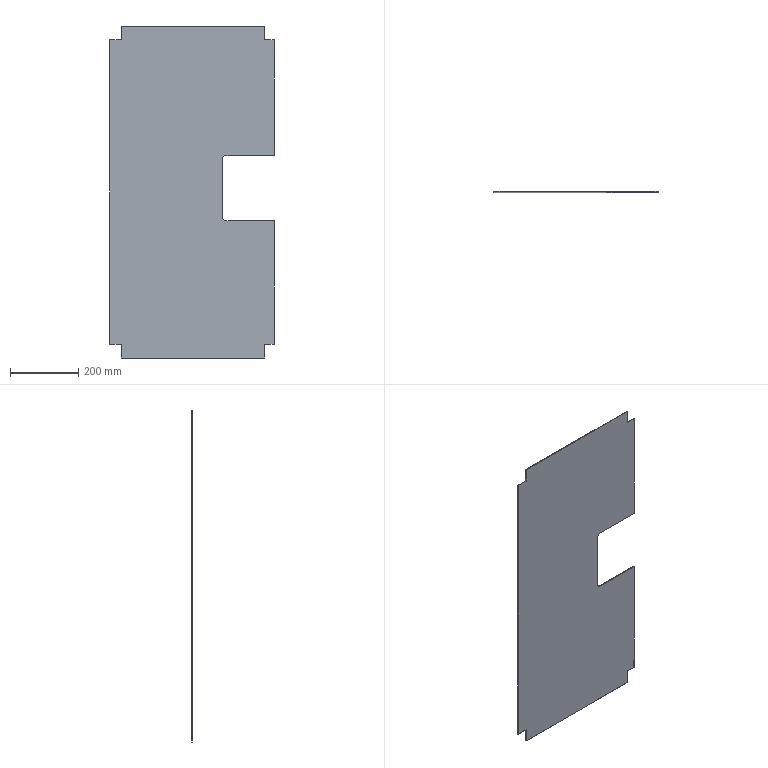Part | SolidWorks | features BaseBody 1 | 1 solid | 20 faces | box 480 x 1.5 x 970 mm | volume 648201 mm3 | plane 18 | cylinder 2 | commonest cylinder face diameters 20 x2
STEP:
#1=CARTESIAN_POINT('',(82.823,-1.5,-83.686));
#2=VERTEX_POINT('',#1);
#3=CARTESIAN_POINT('',(223.5,-1.5,-83.686));
#4=VERTEX_POINT('',#3);
#5=CARTESIAN_POINT('',(0.,-1.5,-83.686));
#6=DIRECTION('',(1.,0.,0.));
#7=VECTOR('',#6,1000.);
#8=LINE('',#5,#7);
#9=EDGE_CURVE('',#2,#4,#8,.T.);
#10=ORIENTED_EDGE('',*,*,#9,.F.);
#11=CARTESIAN_POINT('',(72.823,-1.5,-73.686));
#12=VERTEX_POINT('',#11);
#13=CARTESIAN_POINT('',(82.823,-1.5,-73.686));
#14=DIRECTION('',(0.,-1.,0.));
#15=DIRECTION('',(0.,0.,1.));
#16=AXIS2_PLACEMENT_3D('',#13,#14,#15);
#17=CIRCLE('',#16,10.);
#18=EDGE_CURVE('',#12,#2,#17,.T.);
#19=ORIENTED_EDGE('',*,*,#18,.F.);
#20=CARTESIAN_POINT('',(72.823,-1.5,96.314));
#21=VERTEX_POINT('',#20);
#22=CARTESIAN_POINT('',(72.823,-1.5,0.));
#23=DIRECTION('',(0.,0.,-1.));
#24=VECTOR('',#23,1000.);
#25=LINE('',#22,#24);
#26=EDGE_CURVE('',#21,#12,#25,.T.);
#27=ORIENTED_EDGE('',*,*,#26,.F.);
#28=CARTESIAN_POINT('',(82.823,-1.5,106.314));
#29=VERTEX_POINT('',#28);
#30=CARTESIAN_POINT('',(82.823,-1.5,96.314));
#31=DIRECTION('',(0.,-1.,0.));
#32=DIRECTION('',(0.,0.,1.));
#33=AXIS2_PLACEMENT_3D('',#30,#31,#32);
#34=CIRCLE('',#33,10.);
#35=EDGE_CURVE('',#29,#21,#34,.T.);
#36=ORIENTED_EDGE('',*,*,#35,.F.);
#37=CARTESIAN_POINT('',(223.5,-1.5,106.314));
#38=VERTEX_POINT('',#37);
#39=CARTESIAN_POINT('',(0.,-1.5,106.314));
#40=DIRECTION('',(-1.,0.,0.));
#41=VECTOR('',#40,1000.);
#42=LINE('',#39,#41);
#43=EDGE_CURVE('',#38,#29,#42,.T.);
#44=ORIENTED_EDGE('',*,*,#43,.F.);
#45=CARTESIAN_POINT('',(223.5,-1.5,445.));
#46=VERTEX_POINT('',#45);
#47=CARTESIAN_POINT('',(223.5,-1.5,0.));
#48=DIRECTION('',(0.,0.,-1.));
#49=VECTOR('',#48,1000.);
#50=LINE('',#47,#49);
#51=EDGE_CURVE('',#46,#38,#50,.T.);
#52=ORIENTED_EDGE('',*,*,#51,.F.);
#53=CARTESIAN_POINT('',(195.5,-1.5,445.));
#54=VERTEX_POINT('',#53);
#55=CARTESIAN_POINT('',(0.,-1.5,445.));
#56=DIRECTION('',(1.,0.,0.));
#57=VECTOR('',#56,1000.);
#58=LINE('',#55,#57);
#59=EDGE_CURVE('',#54,#46,#58,.T.);
#60=ORIENTED_EDGE('',*,*,#59,.F.);
#61=CARTESIAN_POINT('',(195.5,-1.5,485.));
#62=VERTEX_POINT('',#61);
#63=CARTESIAN_POINT('',(195.5,-1.5,0.));
#64=DIRECTION('',(0.,0.,-1.));
#65=VECTOR('',#64,1000.);
#66=LINE('',#63,#65);
#67=EDGE_CURVE('',#62,#54,#66,.T.);
#68=ORIENTED_EDGE('',*,*,#67,.F.);
#69=CARTESIAN_POINT('',(-223.5,-1.5,485.));
#70=VERTEX_POINT('',#69);
#71=CARTESIAN_POINT('',(0.,-1.5,485.));
#72=DIRECTION('',(1.,0.,0.));
#73=VECTOR('',#72,1000.);
#74=LINE('',#71,#73);
#75=EDGE_CURVE('',#70,#62,#74,.T.);
#76=ORIENTED_EDGE('',*,*,#75,.F.);
#77=CARTESIAN_POINT('',(-223.5,-1.5,445.));
#78=VERTEX_POINT('',#77);
#79=CARTESIAN_POINT('',(-223.5,-1.5,0.));
#80=DIRECTION('',(0.,0.,1.));
#81=VECTOR('',#80,1000.);
#82=LINE('',#79,#81);
#83=EDGE_CURVE('',#78,#70,#82,.T.);
#84=ORIENTED_EDGE('',*,*,#83,.F.);
#85=CARTESIAN_POINT('',(-256.5,-1.5,445.));
#86=VERTEX_POINT('',#85);
#87=CARTESIAN_POINT('',(0.,-1.5,445.));
#88=DIRECTION('',(1.,0.,0.));
#89=VECTOR('',#88,1000.);
#90=LINE('',#87,#89);
#91=EDGE_CURVE('',#86,#78,#90,.T.);
#92=ORIENTED_EDGE('',*,*,#91,.F.);
#93=CARTESIAN_POINT('',(-256.5,-1.5,-445.));
#94=VERTEX_POINT('',#93);
#95=CARTESIAN_POINT('',(-256.5,-1.5,0.));
#96=DIRECTION('',(0.,0.,1.));
#97=VECTOR('',#96,1000.);
#98=LINE('',#95,#97);
#99=EDGE_CURVE('',#94,#86,#98,.T.);
#100=ORIENTED_EDGE('',*,*,#99,.F.);
#101=CARTESIAN_POINT('',(-223.5,-1.5,-445.));
#102=VERTEX_POINT('',#101);
#103=CARTESIAN_POINT('',(0.,-1.5,-445.));
#104=DIRECTION('',(-1.,0.,0.));
#105=VECTOR('',#104,1000.);
#106=LINE('',#103,#105);
#107=EDGE_CURVE('',#102,#94,#106,.T.);
#108=ORIENTED_EDGE('',*,*,#107,.F.);
#109=CARTESIAN_POINT('',(-223.5,-1.5,-485.));
#110=VERTEX_POINT('',#109);
#111=CARTESIAN_POINT('',(-223.5,-1.5,0.));
#112=DIRECTION('',(0.,0.,1.));
#113=VECTOR('',#112,1000.);
#114=LINE('',#111,#113);
#115=EDGE_CURVE('',#110,#102,#114,.T.);
#116=ORIENTED_EDGE('',*,*,#115,.F.);
#117=CARTESIAN_POINT('',(195.5,-1.5,-485.));
#118=VERTEX_POINT('',#117);
#119=CARTESIAN_POINT('',(0.,-1.5,-485.));
#120=DIRECTION('',(-1.,0.,0.));
#121=VECTOR('',#120,1000.);
#122=LINE('',#119,#121);
#123=EDGE_CURVE('',#118,#110,#122,.T.);
#124=ORIENTED_EDGE('',*,*,#123,.F.);
#125=CARTESIAN_POINT('',(195.5,-1.5,-445.));
#126=VERTEX_POINT('',#125);
#127=CARTESIAN_POINT('',(195.5,-1.5,0.));
#128=DIRECTION('',(0.,0.,-1.));
#129=VECTOR('',#128,1000.);
#130=LINE('',#127,#129);
#131=EDGE_CURVE('',#126,#118,#130,.T.);
#132=ORIENTED_EDGE('',*,*,#131,.F.);
#133=CARTESIAN_POINT('',(223.5,-1.5,-445.));
#134=VERTEX_POINT('',#133);
#135=CARTESIAN_POINT('',(0.,-1.5,-445.));
#136=DIRECTION('',(-1.,0.,0.));
#137=VECTOR('',#136,1000.);
#138=LINE('',#135,#137);
#139=EDGE_CURVE('',#134,#126,#138,.T.);
#140=ORIENTED_EDGE('',*,*,#139,.F.);
#141=CARTESIAN_POINT('',(223.5,-1.5,0.));
#142=DIRECTION('',(0.,0.,-1.));
#143=VECTOR('',#142,1000.);
#144=LINE('',#141,#143);
#145=EDGE_CURVE('',#4,#134,#144,.T.);
#146=ORIENTED_EDGE('',*,*,#145,.F.);
#147=EDGE_LOOP('',(#10,#19,#27,#36,#44,#52,#60,#68,#76,#84,#92,#100,#108,#116,#124,#132,#140,#146));
#148=FACE_OUTER_BOUND('',#147,.T.);
#149=CARTESIAN_POINT('',(0.,-1.5,0.));
#150=DIRECTION('',(0.,1.,0.));
#151=DIRECTION('',(0.,0.,1.));
#152=AXIS2_PLACEMENT_3D('',#149,#150,#151);
#153=PLANE('',#152);
#154=ADVANCED_FACE('',(#148),#153,.F.);
#155=CARTESIAN_POINT('',(223.5,0.,-445.));
#156=VERTEX_POINT('',#155);
#157=CARTESIAN_POINT('',(223.5,-1.5,-445.));
#158=DIRECTION('',(0.,1.,0.));
#159=VECTOR('',#158,1000.);
#160=LINE('',#157,#159);
#161=EDGE_CURVE('',#134,#156,#160,.T.);
#162=ORIENTED_EDGE('',*,*,#161,.T.);
#163=CARTESIAN_POINT('',(223.5,0.,-83.686));
#164=VERTEX_POINT('',#163);
#165=CARTESIAN_POINT('',(223.5,0.,445.));
#166=DIRECTION('',(0.,0.,1.));
#167=VECTOR('',#166,1000.);
#168=LINE('',#165,#167);
#169=EDGE_CURVE('',#156,#164,#168,.T.);
#170=ORIENTED_EDGE('',*,*,#169,.T.);
#171=CARTESIAN_POINT('',(223.5,-1.5,-83.686));
#172=DIRECTION('',(0.,-1.,0.));
#173=VECTOR('',#172,1000.);
#174=LINE('',#171,#173);
#175=EDGE_CURVE('',#164,#4,#174,.T.);
#176=ORIENTED_EDGE('',*,*,#175,.T.);
#177=ORIENTED_EDGE('',*,*,#145,.T.);
#178=EDGE_LOOP('',(#162,#170,#176,#177));
#179=FACE_OUTER_BOUND('',#178,.T.);
#180=CARTESIAN_POINT('',(223.5,-1.5,445.));
#181=DIRECTION('',(1.,0.,0.));
#182=DIRECTION('',(0.,0.,-1.));
#183=AXIS2_PLACEMENT_3D('',#180,#181,#182);
#184=PLANE('',#183);
#185=ADVANCED_FACE('',(#179),#184,.T.);
#186=CARTESIAN_POINT('',(82.823,0.,-83.686));
#187=VERTEX_POINT('',#186);
#188=CARTESIAN_POINT('',(372.823,0.,-83.686));
#189=DIRECTION('',(1.,0.,0.));
#190=VECTOR('',#189,1000.);
#191=LINE('',#188,#190);
#192=EDGE_CURVE('',#187,#164,#191,.T.);
#193=ORIENTED_EDGE('',*,*,#192,.F.);
#194=CARTESIAN_POINT('',(82.823,-10.,-83.686));
#195=DIRECTION('',(0.,1.,0.));
#196=VECTOR('',#195,1000.);
#197=LINE('',#194,#196);
#198=EDGE_CURVE('',#2,#187,#197,.T.);
#199=ORIENTED_EDGE('',*,*,#198,.F.);
#200=ORIENTED_EDGE('',*,*,#9,.T.);
#201=ORIENTED_EDGE('',*,*,#175,.F.);
#202=EDGE_LOOP('',(#193,#199,#200,#201));
#203=FACE_OUTER_BOUND('',#202,.T.);
#204=CARTESIAN_POINT('',(372.823,-10.,-83.686));
#205=DIRECTION('',(0.,0.,-1.));
#206=DIRECTION('',(-1.,0.,0.));
#207=AXIS2_PLACEMENT_3D('',#204,#205,#206);
#208=PLANE('',#207);
#209=ADVANCED_FACE('',(#203),#208,.F.);
#210=CARTESIAN_POINT('',(72.823,0.,-73.686));
#211=VERTEX_POINT('',#210);
#212=CARTESIAN_POINT('',(82.823,0.,-73.686));
#213=DIRECTION('',(0.,-1.,0.));
#214=DIRECTION('',(0.,0.,1.));
#215=AXIS2_PLACEMENT_3D('',#212,#213,#214);
#216=CIRCLE('',#215,10.);
#217=EDGE_CURVE('',#211,#187,#216,.T.);
#218=ORIENTED_EDGE('',*,*,#217,.F.);
#219=CARTESIAN_POINT('',(72.823,-10.,-73.686));
#220=DIRECTION('',(0.,1.,0.));
#221=VECTOR('',#220,1000.);
#222=LINE('',#219,#221);
#223=EDGE_CURVE('',#12,#211,#222,.T.);
#224=ORIENTED_EDGE('',*,*,#223,.F.);
#225=ORIENTED_EDGE('',*,*,#18,.T.);
#226=ORIENTED_EDGE('',*,*,#198,.T.);
#227=EDGE_LOOP('',(#218,#224,#225,#226));
#228=FACE_OUTER_BOUND('',#227,.T.);
#229=CARTESIAN_POINT('',(82.823,-10.,-73.686));
#230=DIRECTION('',(0.,1.,0.));
#231=DIRECTION('',(0.,0.,1.));
#232=AXIS2_PLACEMENT_3D('',#229,#230,#231);
#233=CYLINDRICAL_SURFACE('',#232,10.);
#234=ADVANCED_FACE('',(#228),#233,.F.);
#235=CARTESIAN_POINT('',(72.823,0.,96.314));
#236=VERTEX_POINT('',#235);
#237=CARTESIAN_POINT('',(72.823,0.,-73.686));
#238=DIRECTION('',(0.,0.,-1.));
#239=VECTOR('',#238,1000.);
#240=LINE('',#237,#239);
#241=EDGE_CURVE('',#236,#211,#240,.T.);
#242=ORIENTED_EDGE('',*,*,#241,.F.);
#243=CARTESIAN_POINT('',(72.823,-10.,96.314));
#244=DIRECTION('',(0.,1.,0.));
#245=VECTOR('',#244,1000.);
#246=LINE('',#243,#245);
#247=EDGE_CURVE('',#21,#236,#246,.T.);
#248=ORIENTED_EDGE('',*,*,#247,.F.);
#249=ORIENTED_EDGE('',*,*,#26,.T.);
#250=ORIENTED_EDGE('',*,*,#223,.T.);
#251=EDGE_LOOP('',(#242,#248,#249,#250));
#252=FACE_OUTER_BOUND('',#251,.T.);
#253=CARTESIAN_POINT('',(72.823,-10.,-73.686));
#254=DIRECTION('',(-1.,0.,0.));
#255=DIRECTION('',(0.,0.,1.));
#256=AXIS2_PLACEMENT_3D('',#253,#254,#255);
#257=PLANE('',#256);
#258=ADVANCED_FACE('',(#252),#257,.F.);
#259=CARTESIAN_POINT('',(82.823,0.,106.314));
#260=VERTEX_POINT('',#259);
#261=CARTESIAN_POINT('',(82.823,0.,96.314));
#262=DIRECTION('',(0.,-1.,0.));
#263=DIRECTION('',(0.,0.,1.));
#264=AXIS2_PLACEMENT_3D('',#261,#262,#263);
#265=CIRCLE('',#264,10.);
#266=EDGE_CURVE('',#260,#236,#265,.T.);
#267=ORIENTED_EDGE('',*,*,#266,.F.);
#268=CARTESIAN_POINT('',(82.823,-10.,106.314));
#269=DIRECTION('',(0.,1.,0.));
#270=VECTOR('',#269,1000.);
#271=LINE('',#268,#270);
#272=EDGE_CURVE('',#29,#260,#271,.T.);
#273=ORIENTED_EDGE('',*,*,#272,.F.);
#274=ORIENTED_EDGE('',*,*,#35,.T.);
#275=ORIENTED_EDGE('',*,*,#247,.T.);
#276=EDGE_LOOP('',(#267,#273,#274,#275));
#277=FACE_OUTER_BOUND('',#276,.T.);
#278=CARTESIAN_POINT('',(82.823,-10.,96.314));
#279=DIRECTION('',(0.,1.,0.));
#280=DIRECTION('',(0.,0.,1.));
#281=AXIS2_PLACEMENT_3D('',#278,#279,#280);
#282=CYLINDRICAL_SURFACE('',#281,10.);
#283=ADVANCED_FACE('',(#277),#282,.F.);
#284=ORIENTED_EDGE('',*,*,#43,.T.);
#285=ORIENTED_EDGE('',*,*,#272,.T.);
#286=CARTESIAN_POINT('',(223.5,0.,106.314));
#287=VERTEX_POINT('',#286);
#288=CARTESIAN_POINT('',(82.823,0.,106.314));
#289=DIRECTION('',(-1.,0.,0.));
#290=VECTOR('',#289,1000.);
#291=LINE('',#288,#290);
#292=EDGE_CURVE('',#287,#260,#291,.T.);
#293=ORIENTED_EDGE('',*,*,#292,.F.);
#294=CARTESIAN_POINT('',(223.5,-10.,106.314));
#295=DIRECTION('',(0.,1.,0.));
#296=VECTOR('',#295,1000.);
#297=LINE('',#294,#296);
#298=EDGE_CURVE('',#38,#287,#297,.T.);
#299=ORIENTED_EDGE('',*,*,#298,.F.);
#300=EDGE_LOOP('',(#284,#285,#293,#299));
#301=FACE_OUTER_BOUND('',#300,.T.);
#302=CARTESIAN_POINT('',(82.823,-10.,106.314));
#303=DIRECTION('',(0.,0.,1.));
#304=DIRECTION('',(1.,0.,0.));
#305=AXIS2_PLACEMENT_3D('',#302,#303,#304);
#306=PLANE('',#305);
#307=ADVANCED_FACE('',(#301),#306,.F.);
#308=CARTESIAN_POINT('',(223.5,0.,445.));
#309=VERTEX_POINT('',#308);
#310=CARTESIAN_POINT('',(223.5,-1.5,445.));
#311=DIRECTION('',(0.,-1.,0.));
#312=VECTOR('',#311,1000.);
#313=LINE('',#310,#312);
#314=EDGE_CURVE('',#309,#46,#313,.T.);
#315=ORIENTED_EDGE('',*,*,#314,.T.);
#316=ORIENTED_EDGE('',*,*,#51,.T.);
#317=ORIENTED_EDGE('',*,*,#298,.T.);
#318=CARTESIAN_POINT('',(223.5,0.,445.));
#319=DIRECTION('',(0.,0.,1.));
#320=VECTOR('',#319,1000.);
#321=LINE('',#318,#320);
#322=EDGE_CURVE('',#287,#309,#321,.T.);
#323=ORIENTED_EDGE('',*,*,#322,.T.);
#324=EDGE_LOOP('',(#315,#316,#317,#323));
#325=FACE_OUTER_BOUND('',#324,.T.);
#326=CARTESIAN_POINT('',(223.5,-1.5,445.));
#327=DIRECTION('',(1.,0.,0.));
#328=DIRECTION('',(0.,0.,-1.));
#329=AXIS2_PLACEMENT_3D('',#326,#327,#328);
#330=PLANE('',#329);
#331=ADVANCED_FACE('',(#325),#330,.T.);
#332=ORIENTED_EDGE('',*,*,#59,.T.);
#333=ORIENTED_EDGE('',*,*,#314,.F.);
#334=CARTESIAN_POINT('',(195.5,0.,445.));
#335=VERTEX_POINT('',#334);
#336=CARTESIAN_POINT('',(223.5,0.,445.));
#337=DIRECTION('',(-1.,0.,0.));
#338=VECTOR('',#337,1000.);
#339=LINE('',#336,#338);
#340=EDGE_CURVE('',#309,#335,#339,.T.);
#341=ORIENTED_EDGE('',*,*,#340,.T.);
#342=CARTESIAN_POINT('',(195.5,-1.5,445.));
#343=DIRECTION('',(0.,-1.,0.));
#344=VECTOR('',#343,1000.);
#345=LINE('',#342,#344);
#346=EDGE_CURVE('',#335,#54,#345,.T.);
#347=ORIENTED_EDGE('',*,*,#346,.T.);
#348=EDGE_LOOP('',(#332,#333,#341,#347));
#349=FACE_OUTER_BOUND('',#348,.T.);
#350=CARTESIAN_POINT('',(223.5,-1.5,445.));
#351=DIRECTION('',(0.,0.,1.));
#352=DIRECTION('',(1.,0.,0.));
#353=AXIS2_PLACEMENT_3D('',#350,#351,#352);
#354=PLANE('',#353);
#355=ADVANCED_FACE('',(#349),#354,.T.);
#356=ORIENTED_EDGE('',*,*,#67,.T.);
#357=ORIENTED_EDGE('',*,*,#346,.F.);
#358=CARTESIAN_POINT('',(195.5,0.,485.));
#359=VERTEX_POINT('',#358);
#360=CARTESIAN_POINT('',(195.5,0.,485.));
#361=DIRECTION('',(0.,0.,1.));
#362=VECTOR('',#361,1000.);
#363=LINE('',#360,#362);
#364=EDGE_CURVE('',#335,#359,#363,.T.);
#365=ORIENTED_EDGE('',*,*,#364,.T.);
#366=CARTESIAN_POINT('',(195.5,-1.5,485.));
#367=DIRECTION('',(0.,-1.,0.));
#368=VECTOR('',#367,1000.);
#369=LINE('',#366,#368);
#370=EDGE_CURVE('',#359,#62,#369,.T.);
#371=ORIENTED_EDGE('',*,*,#370,.T.);
#372=EDGE_LOOP('',(#356,#357,#365,#371));
#373=FACE_OUTER_BOUND('',#372,.T.);
#374=CARTESIAN_POINT('',(195.5,-1.5,485.));
#375=DIRECTION('',(1.,0.,0.));
#376=DIRECTION('',(0.,0.,-1.));
#377=AXIS2_PLACEMENT_3D('',#374,#375,#376);
#378=PLANE('',#377);
#379=ADVANCED_FACE('',(#373),#378,.T.);
#380=ORIENTED_EDGE('',*,*,#75,.T.);
#381=ORIENTED_EDGE('',*,*,#370,.F.);
#382=CARTESIAN_POINT('',(-223.5,0.,485.));
#383=VERTEX_POINT('',#382);
#384=CARTESIAN_POINT('',(-223.5,0.,485.));
#385=DIRECTION('',(-1.,0.,0.));
#386=VECTOR('',#385,1000.);
#387=LINE('',#384,#386);
#388=EDGE_CURVE('',#359,#383,#387,.T.);
#389=ORIENTED_EDGE('',*,*,#388,.T.);
#390=CARTESIAN_POINT('',(-223.5,-1.5,485.));
#391=DIRECTION('',(0.,-1.,0.));
#392=VECTOR('',#391,1000.);
#393=LINE('',#390,#392);
#394=EDGE_CURVE('',#383,#70,#393,.T.);
#395=ORIENTED_EDGE('',*,*,#394,.T.);
#396=EDGE_LOOP('',(#380,#381,#389,#395));
#397=FACE_OUTER_BOUND('',#396,.T.);
#398=CARTESIAN_POINT('',(-223.5,-1.5,485.));
#399=DIRECTION('',(0.,0.,1.));
#400=DIRECTION('',(1.,0.,0.));
#401=AXIS2_PLACEMENT_3D('',#398,#399,#400);
#402=PLANE('',#401);
#403=ADVANCED_FACE('',(#397),#402,.T.);
#404=ORIENTED_EDGE('',*,*,#83,.T.);
#405=ORIENTED_EDGE('',*,*,#394,.F.);
#406=CARTESIAN_POINT('',(-223.5,0.,445.));
#407=VERTEX_POINT('',#406);
#408=CARTESIAN_POINT('',(-223.5,0.,485.));
#409=DIRECTION('',(0.,0.,-1.));
#410=VECTOR('',#409,1000.);
#411=LINE('',#408,#410);
#412=EDGE_CURVE('',#383,#407,#411,.T.);
#413=ORIENTED_EDGE('',*,*,#412,.T.);
#414=CARTESIAN_POINT('',(-223.5,-1.5,445.));
#415=DIRECTION('',(0.,-1.,0.));
#416=VECTOR('',#415,1000.);
#417=LINE('',#414,#416);
#418=EDGE_CURVE('',#407,#78,#417,.T.);
#419=ORIENTED_EDGE('',*,*,#418,.T.);
#420=EDGE_LOOP('',(#404,#405,#413,#419));
#421=FACE_OUTER_BOUND('',#420,.T.);
#422=CARTESIAN_POINT('',(-223.5,-1.5,485.));
#423=DIRECTION('',(-1.,0.,0.));
#424=DIRECTION('',(0.,0.,1.));
#425=AXIS2_PLACEMENT_3D('',#422,#423,#424);
#426=PLANE('',#425);
#427=ADVANCED_FACE('',(#421),#426,.T.);
#428=ORIENTED_EDGE('',*,*,#91,.T.);
#429=ORIENTED_EDGE('',*,*,#418,.F.);
#430=CARTESIAN_POINT('',(-256.5,0.,445.));
#431=VERTEX_POINT('',#430);
#432=CARTESIAN_POINT('',(-223.5,0.,445.));
#433=DIRECTION('',(-1.,0.,0.));
#434=VECTOR('',#433,1000.);
#435=LINE('',#432,#434);
#436=EDGE_CURVE('',#407,#431,#435,.T.);
#437=ORIENTED_EDGE('',*,*,#436,.T.);
#438=CARTESIAN_POINT('',(-256.5,-1.5,445.));
#439=DIRECTION('',(0.,-1.,0.));
#440=VECTOR('',#439,1000.);
#441=LINE('',#438,#440);
#442=EDGE_CURVE('',#431,#86,#441,.T.);
#443=ORIENTED_EDGE('',*,*,#442,.T.);
#444=EDGE_LOOP('',(#428,#429,#437,#443));
#445=FACE_OUTER_BOUND('',#444,.T.);
#446=CARTESIAN_POINT('',(-223.5,-1.5,445.));
#447=DIRECTION('',(0.,0.,1.));
#448=DIRECTION('',(1.,0.,0.));
#449=AXIS2_PLACEMENT_3D('',#446,#447,#448);
#450=PLANE('',#449);
#451=ADVANCED_FACE('',(#445),#450,.T.);
#452=ORIENTED_EDGE('',*,*,#99,.T.);
#453=ORIENTED_EDGE('',*,*,#442,.F.);
#454=CARTESIAN_POINT('',(-256.5,0.,-445.));
#455=VERTEX_POINT('',#454);
#456=CARTESIAN_POINT('',(-256.5,0.,445.));
#457=DIRECTION('',(0.,0.,-1.));
#458=VECTOR('',#457,1000.);
#459=LINE('',#456,#458);
#460=EDGE_CURVE('',#431,#455,#459,.T.);
#461=ORIENTED_EDGE('',*,*,#460,.T.);
#462=CARTESIAN_POINT('',(-256.5,-1.5,-445.));
#463=DIRECTION('',(0.,-1.,0.));
#464=VECTOR('',#463,1000.);
#465=LINE('',#462,#464);
#466=EDGE_CURVE('',#455,#94,#465,.T.);
#467=ORIENTED_EDGE('',*,*,#466,.T.);
#468=EDGE_LOOP('',(#452,#453,#461,#467));
#469=FACE_OUTER_BOUND('',#468,.T.);
#470=CARTESIAN_POINT('',(-256.5,-1.5,445.));
#471=DIRECTION('',(-1.,0.,0.));
#472=DIRECTION('',(0.,0.,1.));
#473=AXIS2_PLACEMENT_3D('',#470,#471,#472);
#474=PLANE('',#473);
#475=ADVANCED_FACE('',(#469),#474,.T.);
#476=ORIENTED_EDGE('',*,*,#107,.T.);
#477=ORIENTED_EDGE('',*,*,#466,.F.);
#478=CARTESIAN_POINT('',(-223.5,0.,-445.));
#479=VERTEX_POINT('',#478);
#480=CARTESIAN_POINT('',(-256.5,0.,-445.));
#481=DIRECTION('',(1.,0.,0.));
#482=VECTOR('',#481,1000.);
#483=LINE('',#480,#482);
#484=EDGE_CURVE('',#455,#479,#483,.T.);
#485=ORIENTED_EDGE('',*,*,#484,.T.);
#486=CARTESIAN_POINT('',(-223.5,-1.5,-445.));
#487=DIRECTION('',(0.,-1.,0.));
#488=VECTOR('',#487,1000.);
#489=LINE('',#486,#488);
#490=EDGE_CURVE('',#479,#102,#489,.T.);
#491=ORIENTED_EDGE('',*,*,#490,.T.);
#492=EDGE_LOOP('',(#476,#477,#485,#491));
#493=FACE_OUTER_BOUND('',#492,.T.);
#494=CARTESIAN_POINT('',(-256.5,-1.5,-445.));
#495=DIRECTION('',(0.,0.,-1.));
#496=DIRECTION('',(-1.,0.,0.));
#497=AXIS2_PLACEMENT_3D('',#494,#495,#496);
#498=PLANE('',#497);
#499=ADVANCED_FACE('',(#493),#498,.T.);
#500=ORIENTED_EDGE('',*,*,#115,.T.);
#501=ORIENTED_EDGE('',*,*,#490,.F.);
#502=CARTESIAN_POINT('',(-223.5,0.,-485.));
#503=VERTEX_POINT('',#502);
#504=CARTESIAN_POINT('',(-223.5,0.,-445.));
#505=DIRECTION('',(0.,0.,-1.));
#506=VECTOR('',#505,1000.);
#507=LINE('',#504,#506);
#508=EDGE_CURVE('',#479,#503,#507,.T.);
#509=ORIENTED_EDGE('',*,*,#508,.T.);
#510=CARTESIAN_POINT('',(-223.5,-1.5,-485.));
#511=DIRECTION('',(0.,-1.,0.));
#512=VECTOR('',#511,1000.);
#513=LINE('',#510,#512);
#514=EDGE_CURVE('',#503,#110,#513,.T.);
#515=ORIENTED_EDGE('',*,*,#514,.T.);
#516=EDGE_LOOP('',(#500,#501,#509,#515));
#517=FACE_OUTER_BOUND('',#516,.T.);
#518=CARTESIAN_POINT('',(-223.5,-1.5,-445.));
#519=DIRECTION('',(-1.,0.,0.));
#520=DIRECTION('',(0.,0.,1.));
#521=AXIS2_PLACEMENT_3D('',#518,#519,#520);
#522=PLANE('',#521);
#523=ADVANCED_FACE('',(#517),#522,.T.);
#524=ORIENTED_EDGE('',*,*,#123,.T.);
#525=ORIENTED_EDGE('',*,*,#514,.F.);
#526=CARTESIAN_POINT('',(195.5,0.,-485.));
#527=VERTEX_POINT('',#526);
#528=CARTESIAN_POINT('',(-223.5,0.,-485.));
#529=DIRECTION('',(1.,0.,0.));
#530=VECTOR('',#529,1000.);
#531=LINE('',#528,#530);
#532=EDGE_CURVE('',#503,#527,#531,.T.);
#533=ORIENTED_EDGE('',*,*,#532,.T.);
#534=CARTESIAN_POINT('',(195.5,-1.5,-485.));
#535=DIRECTION('',(0.,-1.,0.));
#536=VECTOR('',#535,1000.);
#537=LINE('',#534,#536);
#538=EDGE_CURVE('',#527,#118,#537,.T.);
#539=ORIENTED_EDGE('',*,*,#538,.T.);
#540=EDGE_LOOP('',(#524,#525,#533,#539));
#541=FACE_OUTER_BOUND('',#540,.T.);
#542=CARTESIAN_POINT('',(-223.5,-1.5,-485.));
#543=DIRECTION('',(0.,0.,-1.));
#544=DIRECTION('',(-1.,0.,0.));
#545=AXIS2_PLACEMENT_3D('',#542,#543,#544);
#546=PLANE('',#545);
#547=ADVANCED_FACE('',(#541),#546,.T.);
#548=ORIENTED_EDGE('',*,*,#131,.T.);
#549=ORIENTED_EDGE('',*,*,#538,.F.);
#550=CARTESIAN_POINT('',(195.5,0.,-445.));
#551=VERTEX_POINT('',#550);
#552=CARTESIAN_POINT('',(195.5,0.,-485.));
#553=DIRECTION('',(0.,0.,1.));
#554=VECTOR('',#553,1000.);
#555=LINE('',#552,#554);
#556=EDGE_CURVE('',#527,#551,#555,.T.);
#557=ORIENTED_EDGE('',*,*,#556,.T.);
#558=CARTESIAN_POINT('',(195.5,-1.5,-445.));
#559=DIRECTION('',(0.,-1.,0.));
#560=VECTOR('',#559,1000.);
#561=LINE('',#558,#560);
#562=EDGE_CURVE('',#551,#126,#561,.T.);
#563=ORIENTED_EDGE('',*,*,#562,.T.);
#564=EDGE_LOOP('',(#548,#549,#557,#563));
#565=FACE_OUTER_BOUND('',#564,.T.);
#566=CARTESIAN_POINT('',(195.5,-1.5,-485.));
#567=DIRECTION('',(1.,0.,0.));
#568=DIRECTION('',(0.,0.,-1.));
#569=AXIS2_PLACEMENT_3D('',#566,#567,#568);
#570=PLANE('',#569);
#571=ADVANCED_FACE('',(#565),#570,.T.);
#572=ORIENTED_EDGE('',*,*,#139,.T.);
#573=ORIENTED_EDGE('',*,*,#562,.F.);
#574=CARTESIAN_POINT('',(223.5,0.,-445.));
#575=DIRECTION('',(1.,0.,0.));
#576=VECTOR('',#575,1000.);
#577=LINE('',#574,#576);
#578=EDGE_CURVE('',#551,#156,#577,.T.);
#579=ORIENTED_EDGE('',*,*,#578,.T.);
#580=ORIENTED_EDGE('',*,*,#161,.F.);
#581=EDGE_LOOP('',(#572,#573,#579,#580));
#582=FACE_OUTER_BOUND('',#581,.T.);
#583=CARTESIAN_POINT('',(223.5,-1.5,-445.));
#584=DIRECTION('',(0.,0.,-1.));
#585=DIRECTION('',(-1.,0.,0.));
#586=AXIS2_PLACEMENT_3D('',#583,#584,#585);
#587=PLANE('',#586);
#588=ADVANCED_FACE('',(#582),#587,.T.);
#589=ORIENTED_EDGE('',*,*,#241,.T.);
#590=ORIENTED_EDGE('',*,*,#217,.T.);
#591=ORIENTED_EDGE('',*,*,#192,.T.);
#592=ORIENTED_EDGE('',*,*,#169,.F.);
#593=ORIENTED_EDGE('',*,*,#578,.F.);
#594=ORIENTED_EDGE('',*,*,#556,.F.);
#595=ORIENTED_EDGE('',*,*,#532,.F.);
#596=ORIENTED_EDGE('',*,*,#508,.F.);
#597=ORIENTED_EDGE('',*,*,#484,.F.);
#598=ORIENTED_EDGE('',*,*,#460,.F.);
#599=ORIENTED_EDGE('',*,*,#436,.F.);
#600=ORIENTED_EDGE('',*,*,#412,.F.);
#601=ORIENTED_EDGE('',*,*,#388,.F.);
#602=ORIENTED_EDGE('',*,*,#364,.F.);
#603=ORIENTED_EDGE('',*,*,#340,.F.);
#604=ORIENTED_EDGE('',*,*,#322,.F.);
#605=ORIENTED_EDGE('',*,*,#292,.T.);
#606=ORIENTED_EDGE('',*,*,#266,.T.);
#607=EDGE_LOOP('',(#589,#590,#591,#592,#593,#594,#595,#596,#597,#598,#599,#600,#601,#602,#603,#604,#605,#606));
#608=FACE_OUTER_BOUND('',#607,.T.);
#609=CARTESIAN_POINT('',(0.,0.,0.));
#610=DIRECTION('',(0.,1.,0.));
#611=DIRECTION('',(0.,0.,1.));
#612=AXIS2_PLACEMENT_3D('',#609,#610,#611);
#613=PLANE('',#612);
#614=ADVANCED_FACE('',(#608),#613,.T.);
#615=CLOSED_SHELL('',(#154,#185,#209,#234,#258,#283,#307,#331,#355,#379,#403,#427,#451,#475,#499,#523,#547,#571,#588,#614));
#616=MANIFOLD_SOLID_BREP('',#615);
#617=CARTESIAN_POINT('',(0.,0.,0.));
#618=DIRECTION('',(0.,0.,1.));
#619=DIRECTION('',(1.,0.,0.));
#620=AXIS2_PLACEMENT_3D('',#617,#618,#619);
#621=(LENGTH_UNIT()NAMED_UNIT(*)SI_UNIT(.MILLI.,.METRE.));
#622=UNCERTAINTY_MEASURE_WITH_UNIT(LENGTH_MEASURE(0.00001),#621,'','');
#623=(NAMED_UNIT(*)PLANE_ANGLE_UNIT()SI_UNIT($,.RADIAN.));
#624=(NAMED_UNIT(*)SI_UNIT($,.STERADIAN.)SOLID_ANGLE_UNIT());
#625=(GEOMETRIC_REPRESENTATION_CONTEXT(3)GLOBAL_UNCERTAINTY_ASSIGNED_CONTEXT((#622))GLOBAL_UNIT_ASSIGNED_CONTEXT((#621,#623,#624))REPRESENTATION_CONTEXT('',''));
#626=ADVANCED_BREP_SHAPE_REPRESENTATION('',(#616,#620),#625);